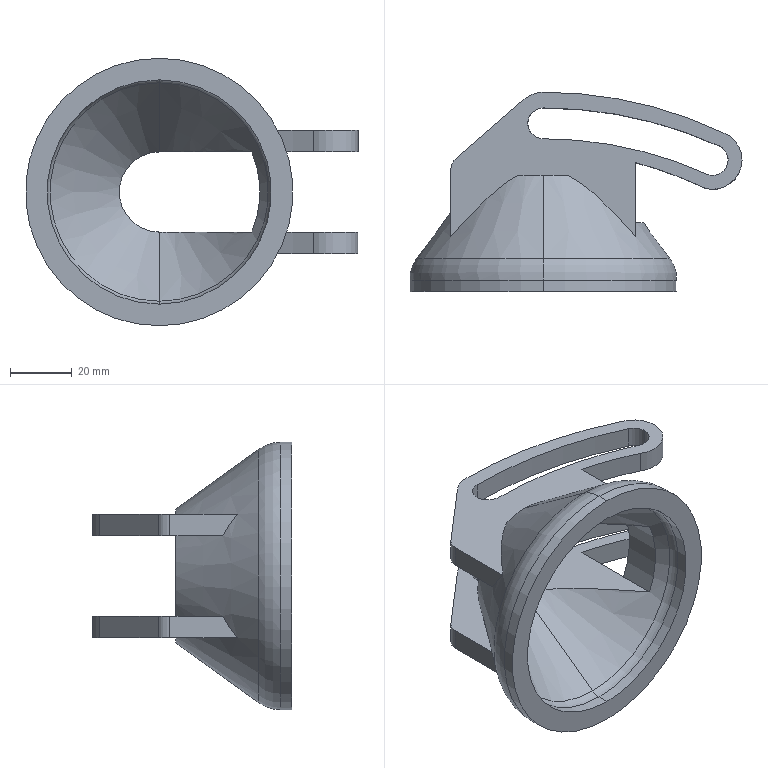Part | SolidWorks | features ICE 5, MirrorPattern 1, Revolution 1 | 1 solid | 48 faces | box 107.891 x 64.658 x 86.78 mm | volume 76040 mm3 | cylinder 26 | plane 14 | torus 4 | cone 4 | commonest cylinder face diameters 10 x8 18.998 x3 19.108 x2 72.78 x2 86.78 x2 237.033 x2